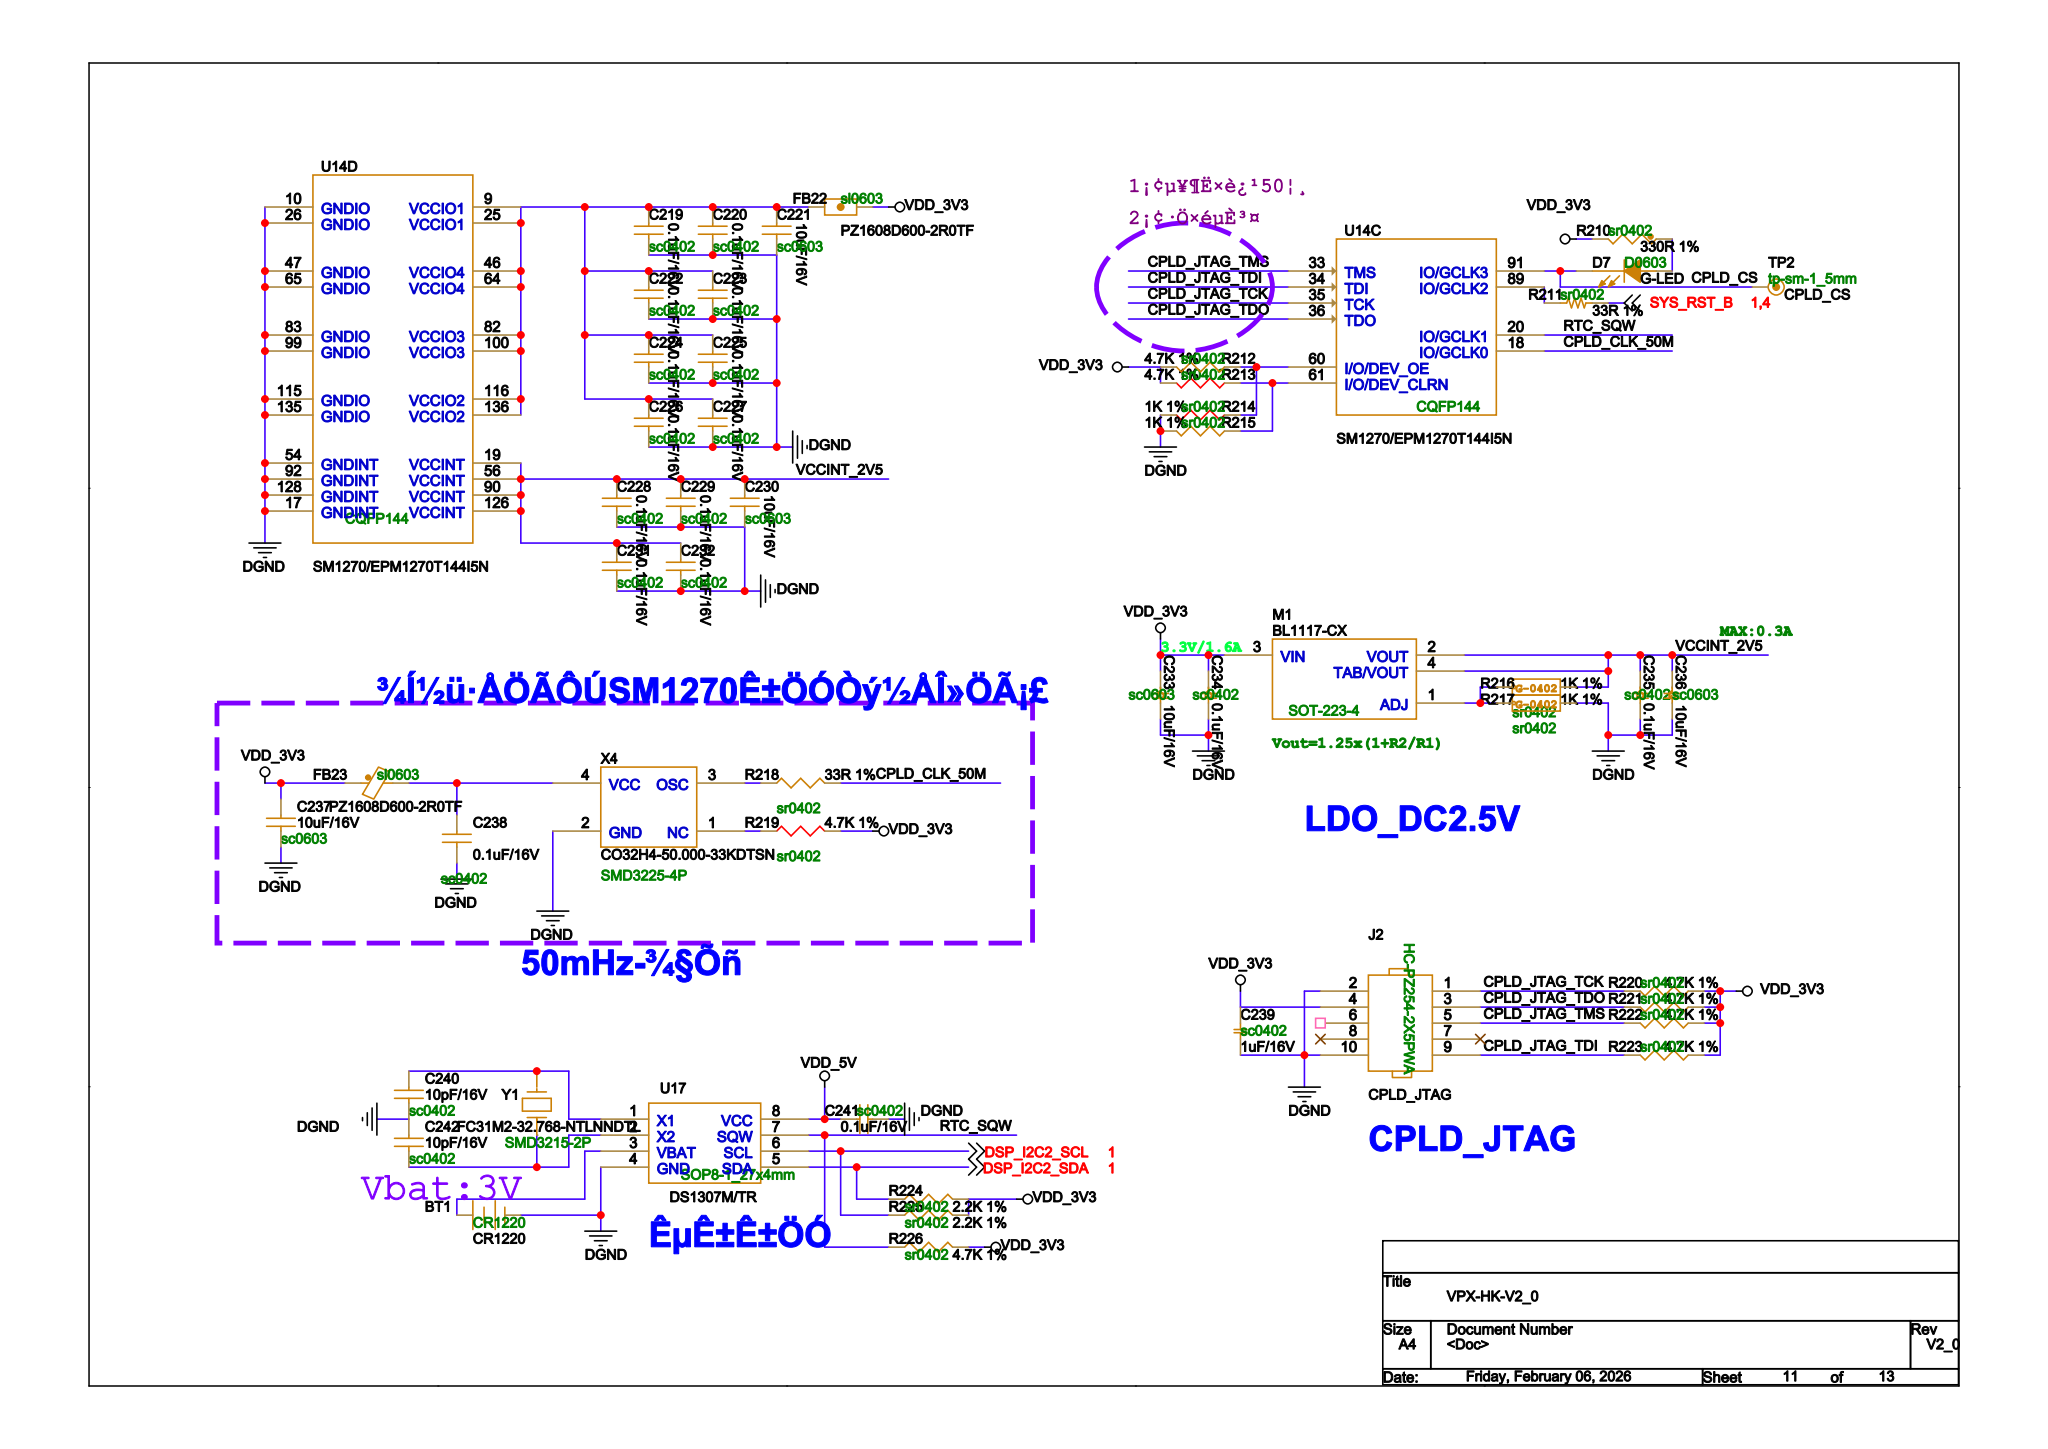Circuit board | Cadence Allegro | 598 parts | 541 nets | one sheet of the schematic
Parts on this sheet (reference | value | footprint):
BT1 | CR1220 | CR1220
C233 | 10uF/16V | SC0603
C234 | 0.1uF/16V | SC0402
C235 | 0.1uF/16V | SC0402
C236 | 10uF/16V | SC0603
C237 | 10uF/16V | SC0603
C238 | 0.1uF/16V | SC0402
C239 | 1uF/16V | SC0402
C240 | 10pF/16V | SC0402
C241 | 0.1uF/16V | SC0402
C242 | 10pF/16V | SC0402
D7 | G-LED | D0603
FB22 | PZ1608D600-2R0TF | SL0603
FB23 | PZ1608D600-2R0TF | SL0603
J2 | CPLD_JTAG | HC-PZ254-2X5PWA
M1 | BL1117-CX | SOT-223-4
R210 | 330R 1% | SR0402
R211 | 33R 1% | SR0402
R218 | 33R 1% | SR0402
R219 | 4.7K 1% | SR0402
R224 | 2.2K 1% | SR0402
R225 | 2.2K 1% | SR0402
R226 | 4.7K 1% | SR0402
TP2 | CPLD_CS | TP-SM-1_5MM
U14 | SM1270/EPM1270T144I5N | CQFP144
U17 | DS1307M/TR | SOP8-1_27X4MM
X4 | CO32H4-50.000-33KDTSN | SMD3225-4P
Y1 | FC31M2-32.768-NTLNNDTL | SMD3215-2P
Nets of these parts (net: part-pin ...):
DGND: BT1-2 C233-2 C234-2 C235-2 C236-2 C237-2 C238-2 C239-2 C240-2 C241-2 C242-1 J2-2 J2-10 U17-4 X4-2 U14-10 U14-17 U14-26 U14-47 U14-54 U14-65 U14-83 U14-92 U14-99 U14-115 U14-128 U14-135
VDD_5V: C241-1 U17-8
CPLD_CLK_50M: R218-2 U14-18
RTC_SQW: R226-2 U17-7 U14-20
N33703255: R211-1 U14-89
CPLD_CS: D7-2 TP2-1 U14-91
CPLD_JTAG_TCK: J2-1 U14-35
CPLD_JTAG_TDI: J2-9 U14-34
CPLD_JTAG_TDO: J2-3 U14-36
CPLD_JTAG_TMS: J2-5 U14-33
VCCINT_2V5: C235-1 C236-1 M1-2 M1-4 U14-19 U14-56 U14-90 U14-126
N33436637: FB22-2 U14-9 U14-25 U14-46 U14-64 U14-82 U14-100 U14-116 U14-136
VDD_3V3: C233-1 C234-1 C237-1 C239-1 FB22-1 FB23-1 J2-4 M1-3 R210-2 R219-2 R224-1 R225-1 R226-1
N33482128: BT1-1 U17-3
SYS_RST_B: R211-2
N33635965: C238-1 FB23-2 X4-4
N33482124: C240-1 U17-1 Y1-2
N33482122: C242-2 U17-2 Y1-1
N33526548: M1-1
DSP_I2C2_SCL: R225-2 U17-6
DSP_I2C2_SDA: R224-2 U17-5
N33635952: R218-1 X4-3
N33635994: R219-1 X4-1
N33703279: D7-1 R210-1